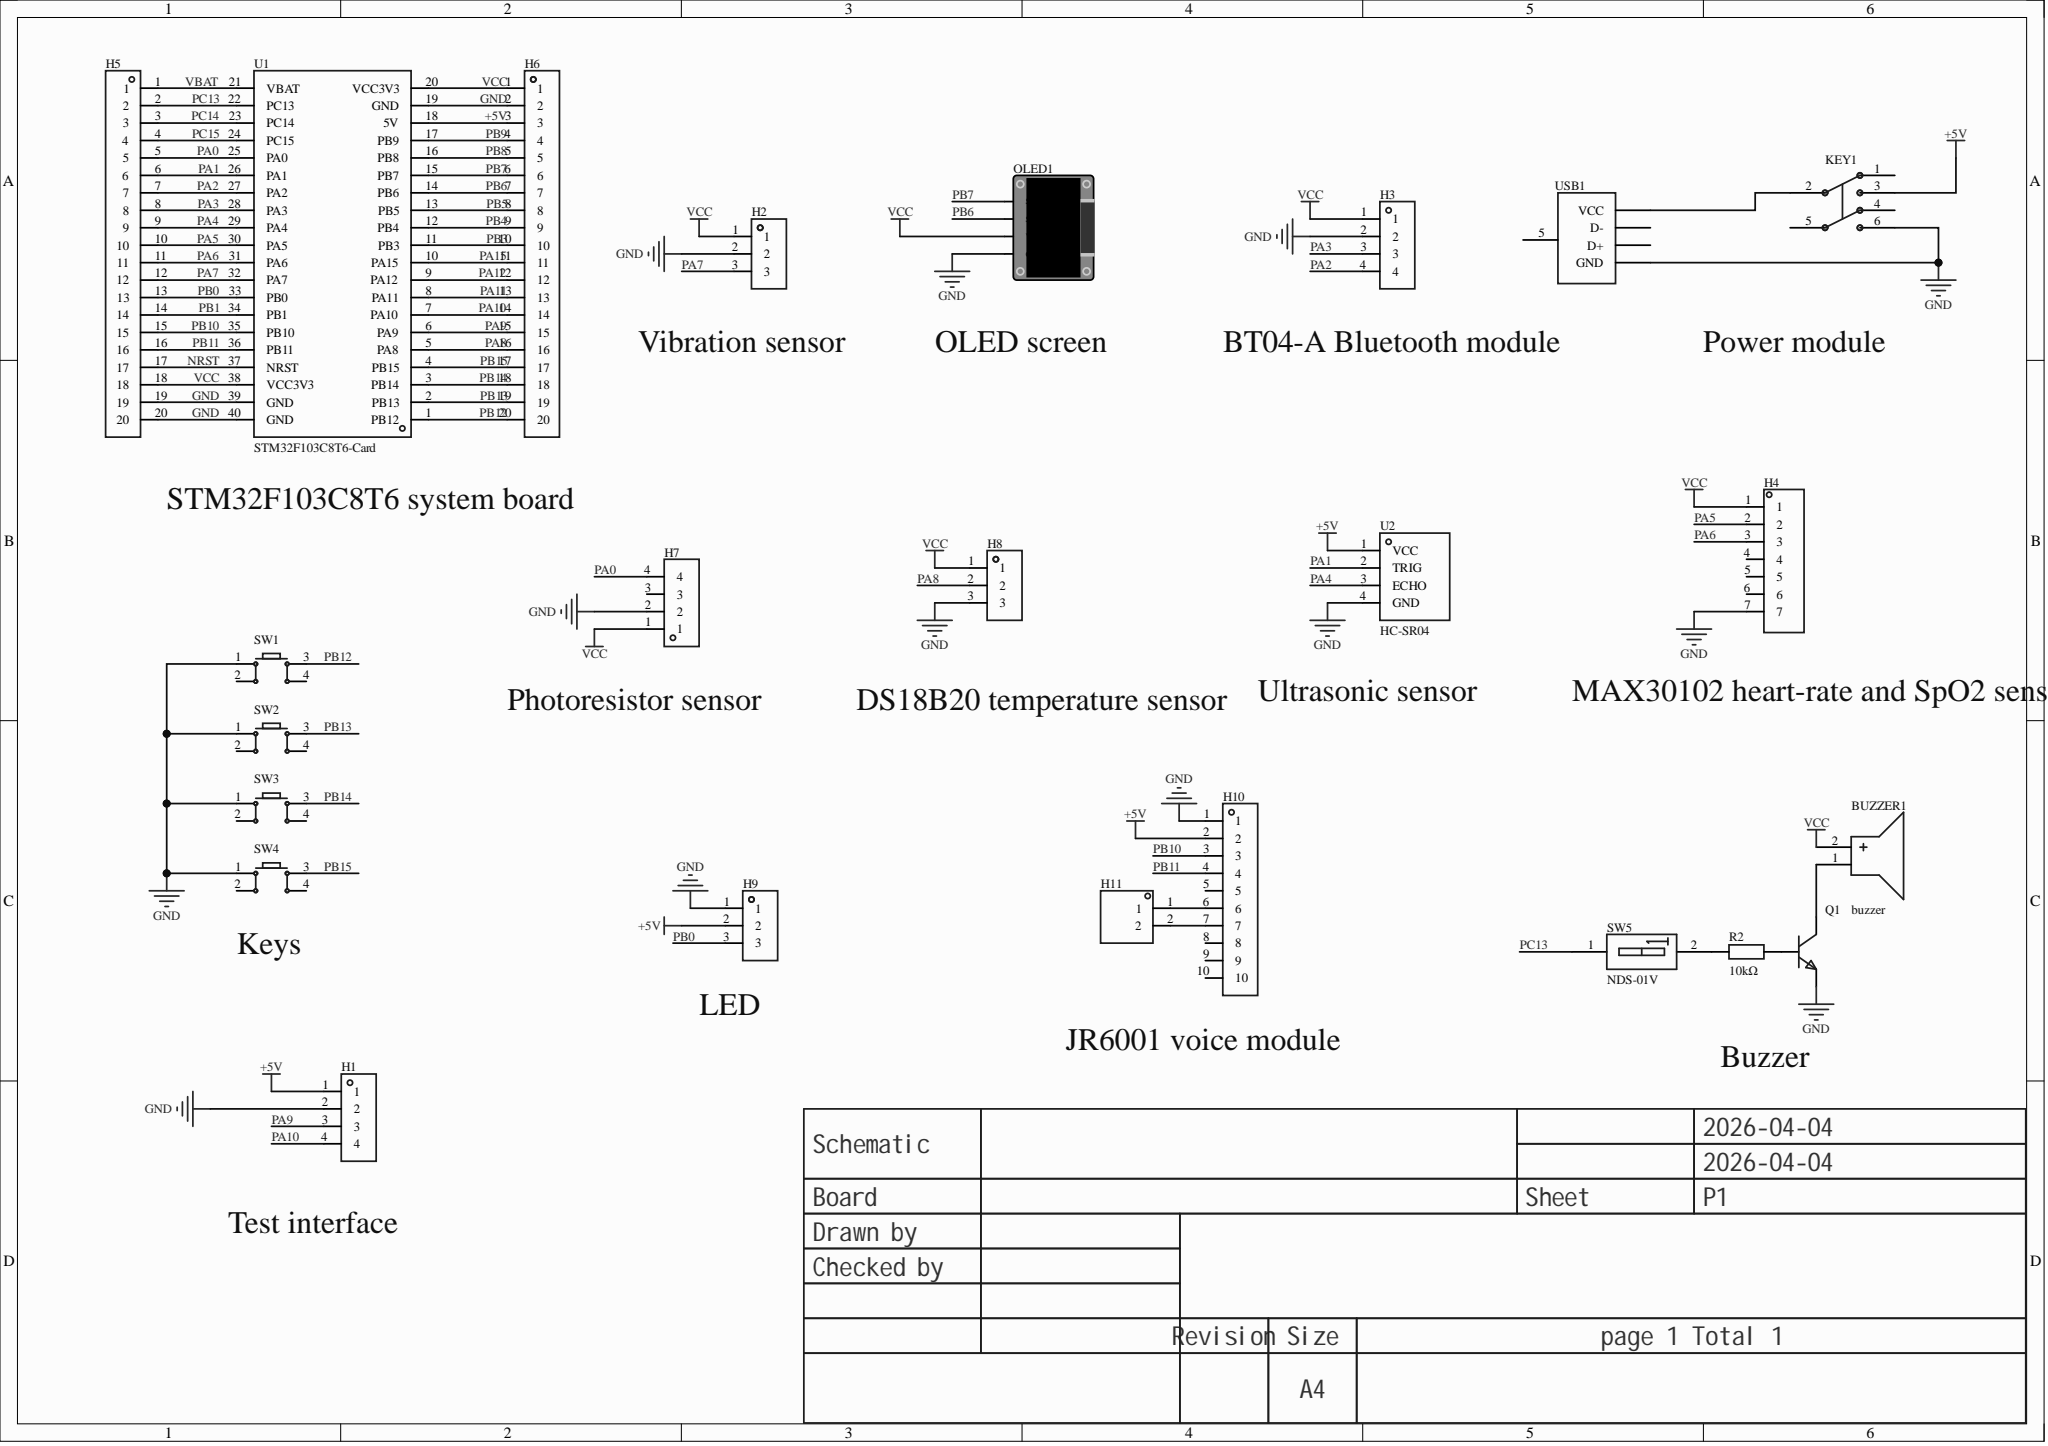Circuit board | Altium Designer | 24 parts | 43 nets
Bill of materials:
Comment,Description,Designator,Footprint,LibRef,Quantity
"buzzer","","BUZZER1","BUZ-TH_BD12.0-P6.00-D0.9-RD","buzzer","1"
"","","H1, H3, H7","HDR-TH_4P-P2.54-V-M","HDR-M_2.54_1x4P","3"
"","","H2, H8, H9","HDR-TH_3P-P2.54-V-F","HDR-F_2.54_1x3P","3"
"","","H4","HDR-TH_7P-P2.54-V-F","HDR-F_2.54_1x7P","1"
"","Pitch:2.54mm;total pins:20;rows:1;pin structure:-;row spacing:-;mounting type:through-hole;round/square pin:-;rated current:-;rated voltage:-;mating pin length:-;plastic height:-;contact material:brass;contact plating:-;colour:black;","H5, H6","HDR-TH_20P-P2.54-V-M-1","HDR-M_2.54_1x20P","2"
"","","H10","HDR-TH_10P-P2.54-V-F","HDR-F_2.54_1x10P","1"
"","","H11","HDR-TH_2P-P2.54-V-M-1","HDR-M_2.54_1x2P","1"
"Non-latching switch 8.5×8.5, silent","6-pin, 8.5×8.5","KEY1","SW-TH_6P-L8.5-W8.5-P2.54","无自锁开关 8.5×8.5 无声","1"
"","","OLED1","0.96OLED_4P","0.96OLED模块_4P","1"
"","","Q1","S8050_TO_92","S8050_TO_NPN","1"
"10kΩ","","R2","Res_1/8W","Res_AXIAL-1/8W","1"
"","","SW1, SW2, SW3, SW4","SW-TH_4P-L6.0-W6.0-P4.50-LS6.5","Key_TH_6x6x6","4"
"NDS-01V","Toggle lever, upright","SW5","SW-TH_2P-L3.9-W9.9-P2.54-LS7.6","NDS-01V_C501305","1"
"STM32F103C8T6-Card","","U1","CONN-TH_L53.3-W22.9_STM32F103C8T6-CARD","STM32F103C8T6-Card","1"
"HC-SR04","","U2","TH_HC-SR04V","HC-SR04","1"
"","","USB1","USB_ Type-B","USB_ Type-B","1"
Netlist (Protel format):
[
BUZZER1
BUZ-TH_BD12.0-P6.00-D0.9-RD
buzzer



]
[
H1
HDR-TH_4P-P2.54-V-M




]
[
H2
HDR-TH_3P-P2.54-V-F




]
[
H3
HDR-TH_4P-P2.54-V-M




]
[
H4
HDR-TH_7P-P2.54-V-F




]
[
H5
HDR-TH_20P-P2.54-V-M-1




]
[
H6
HDR-TH_20P-P2.54-V-M-1




]
[
H7
HDR-TH_4P-P2.54-V-M




]
[
H8
HDR-TH_3P-P2.54-V-F




]
[
H9
HDR-TH_3P-P2.54-V-F




]
[
H10
HDR-TH_10P-P2.54-V-F




]
[
H11
HDR-TH_2P-P2.54-V-M-1




]
[
KEY1
SW-TH_6P-L8.5-W8.5-P2.54
Non-latching switch 8.5×8.5, silent



]
[
OLED1
0.96OLED_4P




]
[
Q1
S8050_TO_92




]
[
R2
Res_1/8W
10kΩ



]
[
SW1
SW-TH_4P-L6.0-W6.0-P4.50-LS6.5




]
[
SW2
SW-TH_4P-L6.0-W6.0-P4.50-LS6.5




]
[
SW3
SW-TH_4P-L6.0-W6.0-P4.50-LS6.5




]
[
SW4
SW-TH_4P-L6.0-W6.0-P4.50-LS6.5




]
[
SW5
SW-TH_2P-L3.9-W9.9-P2.54-LS7.6
NDS-01V



]
[
U1
CONN-TH_L53.3-W22.9_STM32F103C8T6-CARD
STM32F103C8T6-Card



]
[
U2
TH_HC-SR04V
HC-SR04



]
[
USB1
USB_ Type-B




]
(
VCC
BUZZER1-2
H2-1
H3-1
H4-1
H5-18
H6-1
H7-1
H8-1
OLED1-2
U1-20
U1-38
)
(
VBAT
H5-1
U1-21
)
(
PC15
H5-4
U1-24
)
(
PC14
H5-3
U1-23
)
(
PC13
H5-2
SW5-1
U1-22
)
(
PB15
H6-17
SW4-3
U1-4
)
(
PB14
H6-18
SW3-3
U1-3
)
(
PB13
H6-19
SW2-3
U1-2
)
(
PB12
H6-20
SW1-3
U1-1
)
(
PB11
H5-16
H10-4
U1-36
)
(
PB10
H5-15
H10-3
U1-35
)
(
PB9
H6-4
U1-17
)
(
PB8
H6-5
U1-16
)
(
PB7
H6-6
OLED1-4
U1-15
)
(
PB6
H6-7
OLED1-3
U1-14
)
(
PB5
H6-8
U1-13
)
(
PB4
H6-9
U1-12
)
(
PB3
H6-10
U1-11
)
(
PB1
H5-14
U1-34
)
(
PB0
H5-13
H9-3
U1-33
)
(
PA15
H6-11
U1-10
)
(
PA12
H6-12
U1-9
)
(
PA11
H6-13
U1-8
)
(
PA10
H1-4
H6-14
U1-7
)
(
PA9
H1-3
H6-15
U1-6
)
(
PA8
H6-16
H8-2
U1-5
)
(
PA7
H2-3
H5-12
U1-32
)
(
PA6
H4-3
H5-11
U1-31
)
(
PA5
H4-2
H5-10
U1-30
)
(
PA4
H5-9
U1-29
U2-3
)
(
PA3
H3-3
H5-8
U1-28
)
(
PA2
H3-4
H5-7
U1-27
)
(
PA1
H5-6
U1-26
U2-2
)
(
PA0
H5-5
H7-4
U1-25
)
(
NRST
H5-17
U1-37
)
(
NetR2_1
R2-1
SW5-2
)
(
NetQ1_2
Q1-2
R2-2
)
(
NetKEY1_2
KEY1-2
USB1-1
)
(
NetH10_7
H10-7
H11-2
)
(
NetH10_6
H10-6
H11-1
)
(
NetBUZZER1_1
BUZZER1-1
Q1-3
)
(
GND
H1-2
H2-2
H3-2
H4-7
H5-19
H5-20
H6-2
H7-2
H8-3
H9-1
H10-1
KEY1-6
OLED1-1
Q1-1
SW1-1
SW2-1
SW3-1
SW4-1
U1-19
U1-39
U1-40
U2-4
USB1-4
)
(
+5V
H1-1
H6-3
H9-2
H10-2
KEY1-3
U1-18
U2-1
)